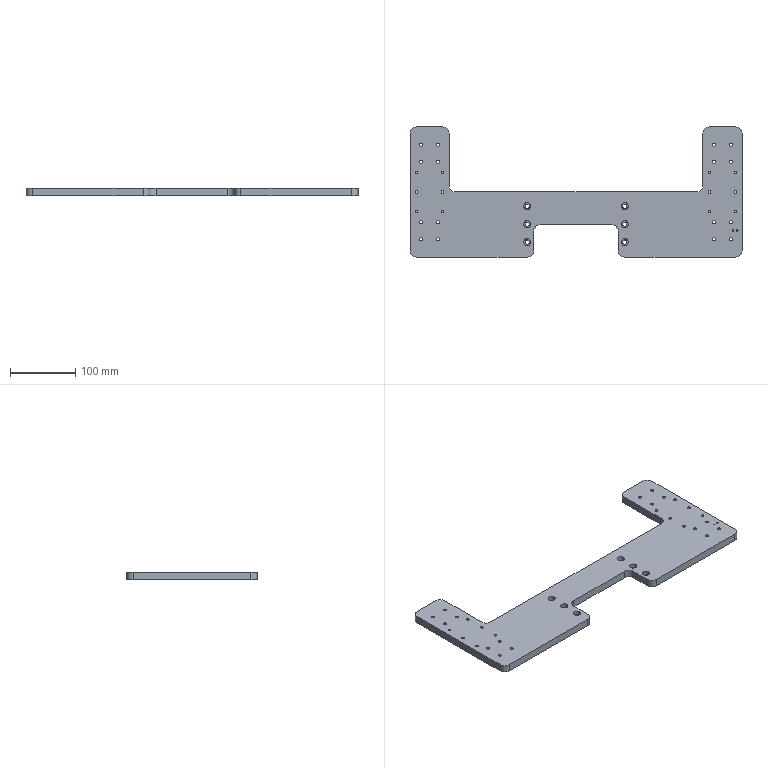Part | STEP file | PN_0002 | 1 solid | 164 faces | box 510 x 200 x 12 mm | volume 664330 mm3 | cylinder 128 | plane 36 | commonest cylinder face diameters 4.5 x32 8 x32 4.2 x24 6.6 x12 11 x12 20 x12